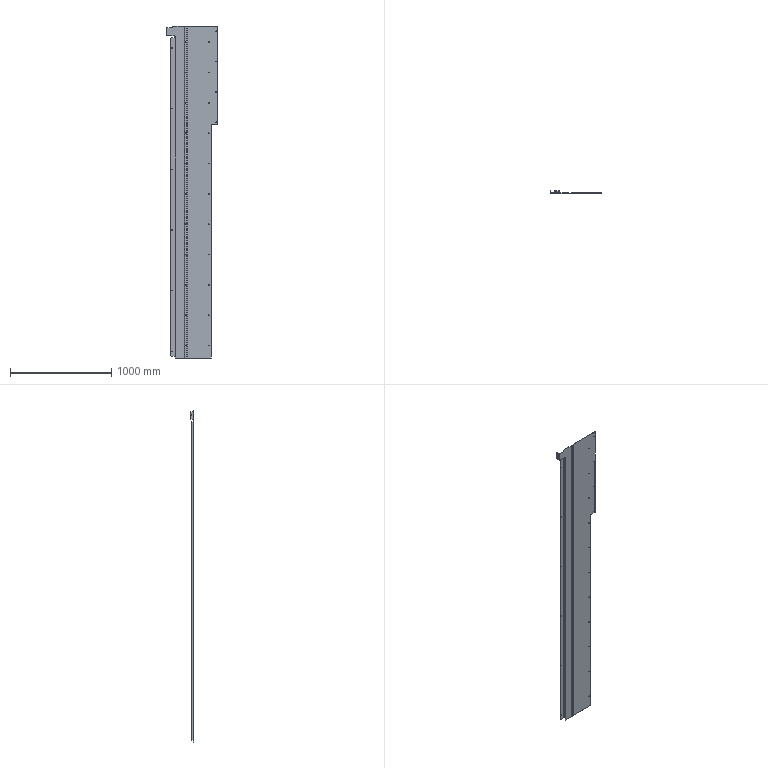Part | STEP file | TS-S88 | 1 solid | 147 faces | box 503 x 33 x 3283 mm | volume 1756521 mm3 | cylinder 87 | plane 60 | commonest cylinder face diameters 5.4 x66 0.4 x7 2.8 x7 10 x3 30 x2 22 x1